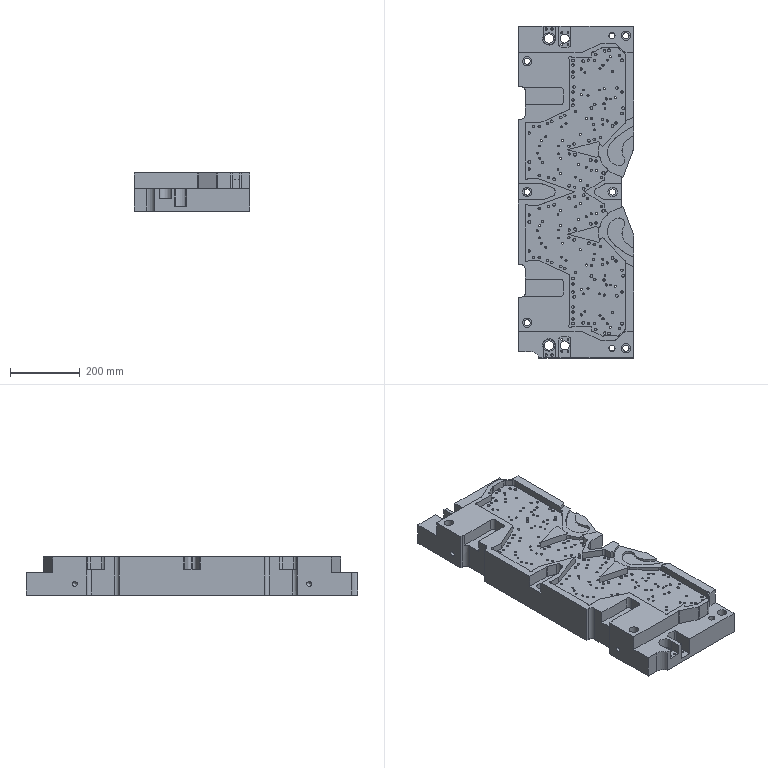Part | NX | features solid 2 | 1 solid | 668 faces | box 330 x 952 x 109.5 mm | volume 26389693 mm3 | cylinder 326 | plane 220 | cone 100 | spline 22 | commonest cylinder face diameters 6.8 x62 8.001 x48 5.2 x42 6.2 x38 8.5 x38 10 x24